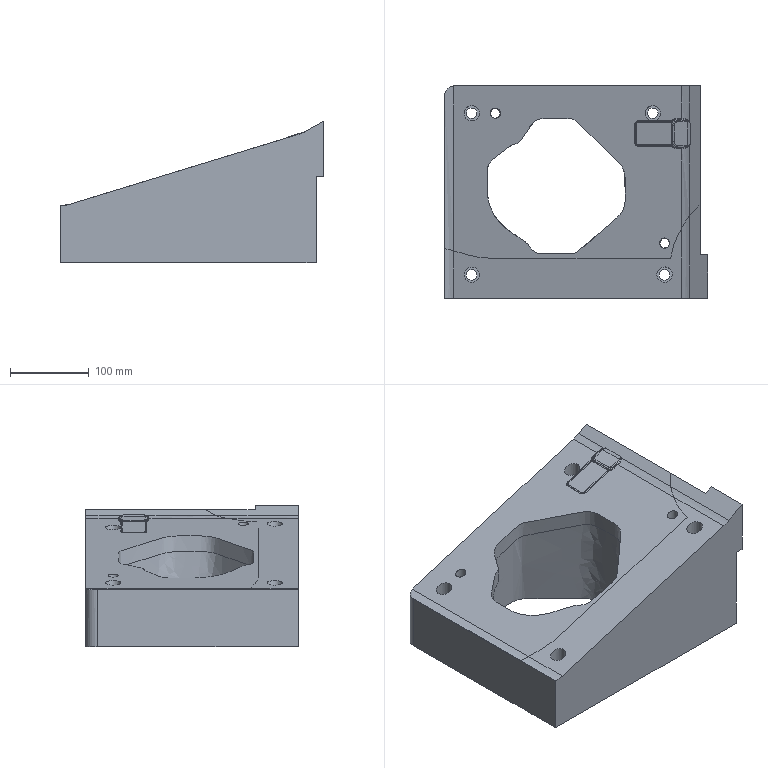Part | NX | features solid 2 | 1 solid | 107 faces | box 335 x 270 x 179.884 mm | volume 7603778 mm3 | spline 80 | plane 14 | cylinder 13 | commonest cylinder face diameters 13.5 x4 19.5 x4 12 x2 13 x2 30 x1